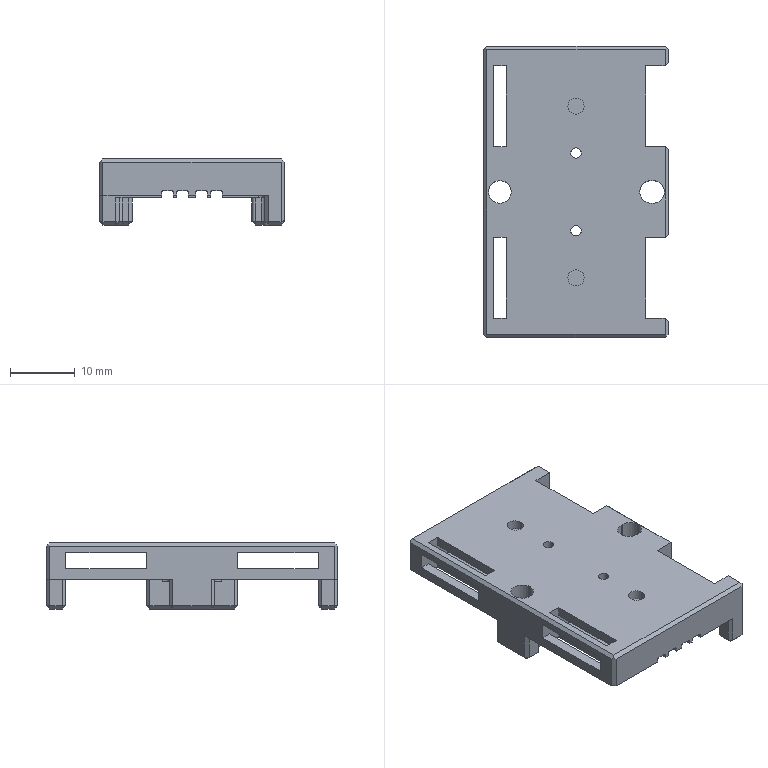Part | SolidWorks | features ICE 49, Chamfer 5, Fillet 3, HoleWzd 2, Cut 1, DelFace 1, Extrusion 1 | 1 solid | 209 faces | box 28.5 x 45 x 10.2 mm | volume 4918 mm3 | plane 154 | cylinder 47 | cone 8 | commonest cylinder face diameters 0.3 x8 0.6 x8 1 x8 2.2 x8 3.5 x5 1.6 x4